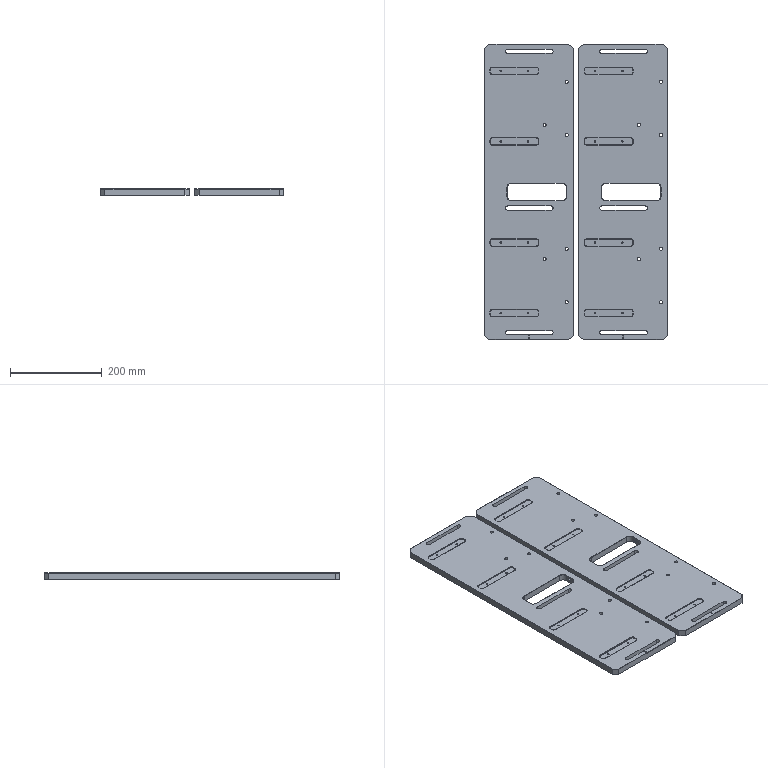Part | 2 solids | 264 faces | box 401 x 645 x 14 mm | volume 3268100 mm3 | plane 142 | cylinder 82 | cone 40 | commonest cylinder face diameters 10 x32 3.2 x16 6.8 x14 9 x12 20 x8